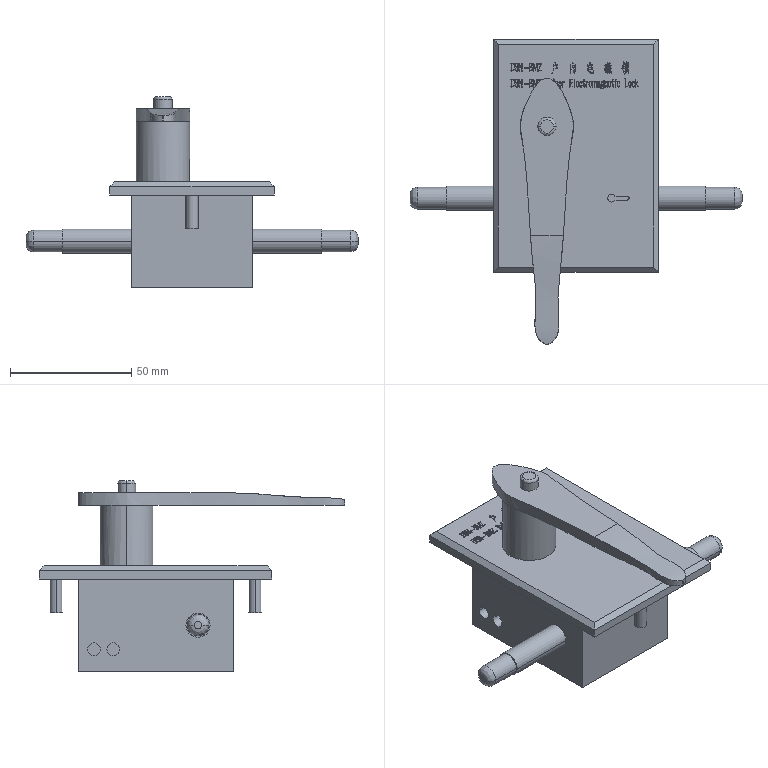Part | STEP file | DSN-BMZ indoor electromagnetic lock | 1 solid | 1367 faces | box 137 x 126 x 78.5 mm | volume 180321 mm3 | plane 852 | spline 486 | cylinder 23 | other 4 | torus 2 | commonest cylinder face diameters 5 x4 5.3 x4 9 x4 10 x4 1.582 x2 7.5 x2